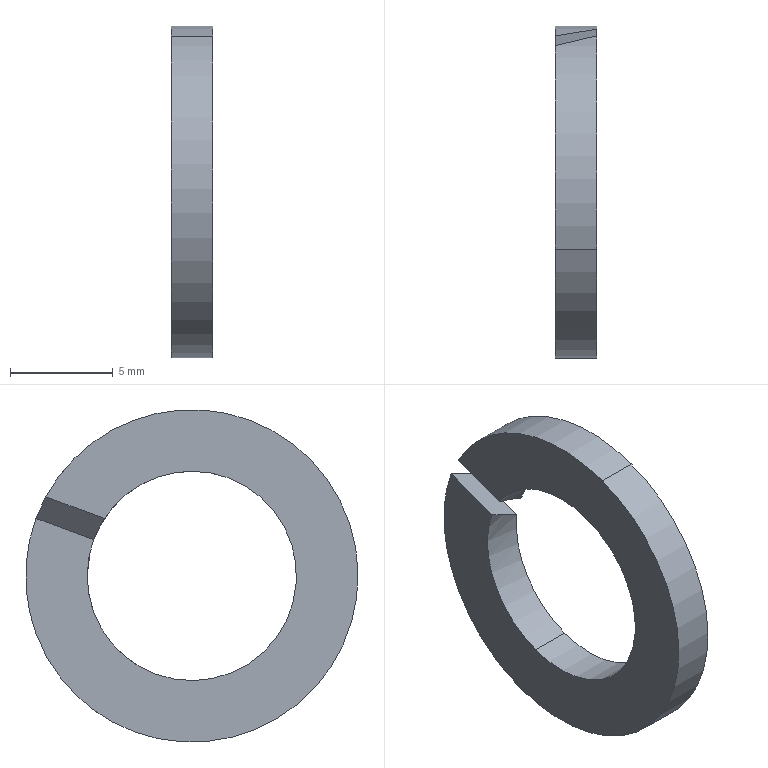Part | SolidWorks | features BaseBody 1 | 1 solid | 10 faces | box 2 x 16.2 x 16.2 mm | volume 241.867 mm3 | cylinder 6 | plane 4 | commonest cylinder face diameters 10.2 x3 16.2 x3
STEP:
#1=CARTESIAN_POINT('',(456.1,149.784,-28.234));
#2=VERTEX_POINT('',#1);
#3=CARTESIAN_POINT('',(456.1,146.766,-34.784));
#4=VERTEX_POINT('',#3);
#5=CARTESIAN_POINT('',(456.1,145.,-30.));
#6=DIRECTION('',(-1.,0.,0.));
#7=DIRECTION('',(0.,-0.3463,0.9381));
#8=AXIS2_PLACEMENT_3D('',#5,#6,#7);
#9=CIRCLE('',#8,5.1);
#10=EDGE_CURVE('',#2,#4,#9,.T.);
#11=ORIENTED_EDGE('',*,*,#10,.T.);
#12=CARTESIAN_POINT('',(458.1,146.766,-34.784));
#13=VERTEX_POINT('',#12);
#14=CARTESIAN_POINT('',(456.1,146.766,-34.784));
#15=DIRECTION('',(1.,0.,0.));
#16=VECTOR('',#15,1000.);
#17=LINE('',#14,#16);
#18=EDGE_CURVE('',#4,#13,#17,.T.);
#19=ORIENTED_EDGE('',*,*,#18,.T.);
#20=CARTESIAN_POINT('',(458.1,150.06,-29.363));
#21=VERTEX_POINT('',#20);
#22=CARTESIAN_POINT('',(458.1,145.,-30.));
#23=DIRECTION('',(-1.,0.,0.));
#24=DIRECTION('',(0.,0.3463,-0.9381));
#25=AXIS2_PLACEMENT_3D('',#22,#23,#24);
#26=CIRCLE('',#25,5.1);
#27=EDGE_CURVE('',#21,#13,#26,.T.);
#28=ORIENTED_EDGE('',*,*,#27,.F.);
#29=CARTESIAN_POINT('',(458.1,150.06,-29.363));
#30=CARTESIAN_POINT('',(457.444,150.011,-28.977));
#31=CARTESIAN_POINT('',(456.774,149.919,-28.599));
#32=CARTESIAN_POINT('',(456.1,149.784,-28.234));
#33=(BOUNDED_CURVE()B_SPLINE_CURVE(3,(#29,#30,#31,#32),.UNSPECIFIED.,.F.,.T.)B_SPLINE_CURVE_WITH_KNOTS((4,4),(1.342,1.571),.UNSPECIFIED.)CURVE()GEOMETRIC_REPRESENTATION_ITEM()RATIONAL_B_SPLINE_CURVE((1.,0.9957,0.9957,1.))REPRESENTATION_ITEM(''));
#34=EDGE_CURVE('',#21,#2,#33,.T.);
#35=ORIENTED_EDGE('',*,*,#34,.T.);
#36=EDGE_LOOP('',(#11,#19,#28,#35));
#37=FACE_OUTER_BOUND('',#36,.T.);
#38=CARTESIAN_POINT('',(456.1,145.,-30.));
#39=DIRECTION('',(1.,0.,0.));
#40=DIRECTION('',(0.,-0.3463,0.9381));
#41=AXIS2_PLACEMENT_3D('',#38,#39,#40);
#42=CYLINDRICAL_SURFACE('',#41,5.1);
#43=ADVANCED_FACE('',(#37),#42,.F.);
#44=ORIENTED_EDGE('',*,*,#18,.F.);
#45=CARTESIAN_POINT('',(456.1,143.234,-25.216));
#46=VERTEX_POINT('',#45);
#47=CARTESIAN_POINT('',(456.1,145.,-30.));
#48=DIRECTION('',(-1.,0.,0.));
#49=DIRECTION('',(0.,-0.3463,0.9381));
#50=AXIS2_PLACEMENT_3D('',#47,#48,#49);
#51=CIRCLE('',#50,5.1);
#52=EDGE_CURVE('',#4,#46,#51,.T.);
#53=ORIENTED_EDGE('',*,*,#52,.T.);
#54=CARTESIAN_POINT('',(458.1,143.234,-25.216));
#55=VERTEX_POINT('',#54);
#56=CARTESIAN_POINT('',(456.1,143.234,-25.216));
#57=DIRECTION('',(1.,0.,0.));
#58=VECTOR('',#57,1000.);
#59=LINE('',#56,#58);
#60=EDGE_CURVE('',#46,#55,#59,.T.);
#61=ORIENTED_EDGE('',*,*,#60,.T.);
#62=CARTESIAN_POINT('',(458.1,145.,-30.));
#63=DIRECTION('',(-1.,0.,0.));
#64=DIRECTION('',(0.,0.3463,-0.9381));
#65=AXIS2_PLACEMENT_3D('',#62,#63,#64);
#66=CIRCLE('',#65,5.1);
#67=EDGE_CURVE('',#13,#55,#66,.T.);
#68=ORIENTED_EDGE('',*,*,#67,.F.);
#69=EDGE_LOOP('',(#44,#53,#61,#68));
#70=FACE_OUTER_BOUND('',#69,.T.);
#71=CARTESIAN_POINT('',(456.1,145.,-30.));
#72=DIRECTION('',(1.,0.,0.));
#73=DIRECTION('',(0.,-0.3463,0.9381));
#74=AXIS2_PLACEMENT_3D('',#71,#72,#73);
#75=CYLINDRICAL_SURFACE('',#74,5.1);
#76=ADVANCED_FACE('',(#70),#75,.F.);
#77=CARTESIAN_POINT('',(456.1,147.805,-37.599));
#78=VERTEX_POINT('',#77);
#79=CARTESIAN_POINT('',(456.1,142.195,-22.401));
#80=VERTEX_POINT('',#79);
#81=CARTESIAN_POINT('',(456.1,145.,-30.));
#82=DIRECTION('',(-1.,0.,0.));
#83=DIRECTION('',(0.,-0.3463,0.9381));
#84=AXIS2_PLACEMENT_3D('',#81,#82,#83);
#85=CIRCLE('',#84,8.1);
#86=EDGE_CURVE('',#78,#80,#85,.T.);
#87=ORIENTED_EDGE('',*,*,#86,.F.);
#88=CARTESIAN_POINT('',(458.1,147.805,-37.599));
#89=VERTEX_POINT('',#88);
#90=CARTESIAN_POINT('',(456.1,147.805,-37.599));
#91=DIRECTION('',(1.,0.,0.));
#92=VECTOR('',#91,1000.);
#93=LINE('',#90,#92);
#94=EDGE_CURVE('',#78,#89,#93,.T.);
#95=ORIENTED_EDGE('',*,*,#94,.T.);
#96=CARTESIAN_POINT('',(458.1,142.195,-22.401));
#97=VERTEX_POINT('',#96);
#98=CARTESIAN_POINT('',(458.1,145.,-30.));
#99=DIRECTION('',(-1.,0.,0.));
#100=DIRECTION('',(0.,0.3463,-0.9381));
#101=AXIS2_PLACEMENT_3D('',#98,#99,#100);
#102=CIRCLE('',#101,8.1);
#103=EDGE_CURVE('',#89,#97,#102,.T.);
#104=ORIENTED_EDGE('',*,*,#103,.T.);
#105=CARTESIAN_POINT('',(456.1,142.195,-22.401));
#106=DIRECTION('',(1.,0.,0.));
#107=VECTOR('',#106,1000.);
#108=LINE('',#105,#107);
#109=EDGE_CURVE('',#80,#97,#108,.T.);
#110=ORIENTED_EDGE('',*,*,#109,.F.);
#111=EDGE_LOOP('',(#87,#95,#104,#110));
#112=FACE_OUTER_BOUND('',#111,.T.);
#113=CARTESIAN_POINT('',(456.1,145.,-30.));
#114=DIRECTION('',(1.,0.,0.));
#115=DIRECTION('',(0.,-0.3463,0.9381));
#116=AXIS2_PLACEMENT_3D('',#113,#114,#115);
#117=CYLINDRICAL_SURFACE('',#116,8.1);
#118=ADVANCED_FACE('',(#112),#117,.T.);
#119=CARTESIAN_POINT('',(456.1,152.121,-26.14));
#120=VERTEX_POINT('',#119);
#121=CARTESIAN_POINT('',(456.1,145.,-30.));
#122=DIRECTION('',(-1.,0.,0.));
#123=DIRECTION('',(0.,-0.3463,0.9381));
#124=AXIS2_PLACEMENT_3D('',#121,#122,#123);
#125=CIRCLE('',#124,8.1);
#126=EDGE_CURVE('',#80,#120,#125,.T.);
#127=ORIENTED_EDGE('',*,*,#126,.F.);
#128=ORIENTED_EDGE('',*,*,#109,.T.);
#129=CARTESIAN_POINT('',(458.1,152.599,-27.195));
#130=VERTEX_POINT('',#129);
#131=CARTESIAN_POINT('',(458.1,145.,-30.));
#132=DIRECTION('',(-1.,0.,0.));
#133=DIRECTION('',(0.,0.3463,-0.9381));
#134=AXIS2_PLACEMENT_3D('',#131,#132,#133);
#135=CIRCLE('',#134,8.1);
#136=EDGE_CURVE('',#97,#130,#135,.T.);
#137=ORIENTED_EDGE('',*,*,#136,.T.);
#138=CARTESIAN_POINT('',(456.1,152.121,-26.14));
#139=CARTESIAN_POINT('',(456.763,152.305,-26.48));
#140=CARTESIAN_POINT('',(457.43,152.465,-26.832));
#141=CARTESIAN_POINT('',(458.1,152.599,-27.195));
#142=(BOUNDED_CURVE()B_SPLINE_CURVE(3,(#138,#139,#140,#141),.UNSPECIFIED.,.F.,.F.)B_SPLINE_CURVE_WITH_KNOTS((4,4),(4.569,4.712),.UNSPECIFIED.)CURVE()GEOMETRIC_REPRESENTATION_ITEM()RATIONAL_B_SPLINE_CURVE((1.,0.9983,0.9983,1.))REPRESENTATION_ITEM(''));
#143=EDGE_CURVE('',#120,#130,#142,.T.);
#144=ORIENTED_EDGE('',*,*,#143,.F.);
#145=EDGE_LOOP('',(#127,#128,#137,#144));
#146=FACE_OUTER_BOUND('',#145,.T.);
#147=CARTESIAN_POINT('',(456.1,145.,-30.));
#148=DIRECTION('',(1.,0.,0.));
#149=DIRECTION('',(0.,-0.3463,0.9381));
#150=AXIS2_PLACEMENT_3D('',#147,#148,#149);
#151=CYLINDRICAL_SURFACE('',#150,8.1);
#152=ADVANCED_FACE('',(#146),#151,.T.);
#153=ORIENTED_EDGE('',*,*,#10,.F.);
#154=CARTESIAN_POINT('',(456.1,152.599,-27.195));
#155=VERTEX_POINT('',#154);
#156=CARTESIAN_POINT('',(456.1,152.6,-27.194));
#157=DIRECTION('',(0.,-0.9381,-0.3463));
#158=VECTOR('',#157,1000.);
#159=LINE('',#156,#158);
#160=EDGE_CURVE('',#155,#2,#159,.T.);
#161=ORIENTED_EDGE('',*,*,#160,.F.);
#162=CARTESIAN_POINT('',(456.1,145.,-30.));
#163=DIRECTION('',(-1.,0.,0.));
#164=DIRECTION('',(0.,-0.3463,0.9381));
#165=AXIS2_PLACEMENT_3D('',#162,#163,#164);
#166=CIRCLE('',#165,8.1);
#167=EDGE_CURVE('',#155,#78,#166,.T.);
#168=ORIENTED_EDGE('',*,*,#167,.T.);
#169=ORIENTED_EDGE('',*,*,#86,.T.);
#170=ORIENTED_EDGE('',*,*,#126,.T.);
#171=CARTESIAN_POINT('',(456.1,149.26,-27.196));
#172=VERTEX_POINT('',#171);
#173=CARTESIAN_POINT('',(456.1,152.2,-26.111));
#174=DIRECTION('',(0.,-0.9381,-0.3463));
#175=VECTOR('',#174,1000.);
#176=LINE('',#173,#175);
#177=EDGE_CURVE('',#120,#172,#176,.T.);
#178=ORIENTED_EDGE('',*,*,#177,.T.);
#179=CARTESIAN_POINT('',(456.1,145.,-30.));
#180=DIRECTION('',(-1.,0.,0.));
#181=DIRECTION('',(0.,-0.3463,0.9381));
#182=AXIS2_PLACEMENT_3D('',#179,#180,#181);
#183=CIRCLE('',#182,5.1);
#184=EDGE_CURVE('',#46,#172,#183,.T.);
#185=ORIENTED_EDGE('',*,*,#184,.F.);
#186=ORIENTED_EDGE('',*,*,#52,.F.);
#187=EDGE_LOOP('',(#153,#161,#168,#169,#170,#178,#185,#186));
#188=FACE_OUTER_BOUND('',#187,.T.);
#189=CARTESIAN_POINT('',(456.1,145.,-30.));
#190=DIRECTION('',(1.,0.,0.));
#191=DIRECTION('',(0.,-0.3463,0.9381));
#192=AXIS2_PLACEMENT_3D('',#189,#190,#191);
#193=PLANE('',#192);
#194=ADVANCED_FACE('',(#188),#193,.F.);
#195=CARTESIAN_POINT('',(458.1,152.921,-28.306));
#196=VERTEX_POINT('',#195);
#197=CARTESIAN_POINT('',(458.1,153.,-28.277));
#198=DIRECTION('',(0.,-0.9381,-0.3463));
#199=VECTOR('',#198,1000.);
#200=LINE('',#197,#199);
#201=EDGE_CURVE('',#196,#21,#200,.T.);
#202=ORIENTED_EDGE('',*,*,#201,.T.);
#203=ORIENTED_EDGE('',*,*,#27,.T.);
#204=ORIENTED_EDGE('',*,*,#67,.T.);
#205=CARTESIAN_POINT('',(458.1,149.784,-28.234));
#206=VERTEX_POINT('',#205);
#207=CARTESIAN_POINT('',(458.1,145.,-30.));
#208=DIRECTION('',(-1.,0.,0.));
#209=DIRECTION('',(0.,0.3463,-0.9381));
#210=AXIS2_PLACEMENT_3D('',#207,#208,#209);
#211=CIRCLE('',#210,5.1);
#212=EDGE_CURVE('',#55,#206,#211,.T.);
#213=ORIENTED_EDGE('',*,*,#212,.T.);
#214=CARTESIAN_POINT('',(458.1,152.6,-27.194));
#215=DIRECTION('',(0.,-0.9381,-0.3463));
#216=VECTOR('',#215,1000.);
#217=LINE('',#214,#216);
#218=EDGE_CURVE('',#130,#206,#217,.T.);
#219=ORIENTED_EDGE('',*,*,#218,.F.);
#220=ORIENTED_EDGE('',*,*,#136,.F.);
#221=ORIENTED_EDGE('',*,*,#103,.F.);
#222=CARTESIAN_POINT('',(458.1,145.,-30.));
#223=DIRECTION('',(-1.,0.,0.));
#224=DIRECTION('',(0.,0.3463,-0.9381));
#225=AXIS2_PLACEMENT_3D('',#222,#223,#224);
#226=CIRCLE('',#225,8.1);
#227=EDGE_CURVE('',#196,#89,#226,.T.);
#228=ORIENTED_EDGE('',*,*,#227,.F.);
#229=EDGE_LOOP('',(#202,#203,#204,#213,#219,#220,#221,#228));
#230=FACE_OUTER_BOUND('',#229,.T.);
#231=CARTESIAN_POINT('',(458.1,145.,-30.));
#232=DIRECTION('',(1.,0.,0.));
#233=DIRECTION('',(0.,-0.3463,0.9381));
#234=AXIS2_PLACEMENT_3D('',#231,#232,#233);
#235=PLANE('',#234);
#236=ADVANCED_FACE('',(#230),#235,.T.);
#237=ORIENTED_EDGE('',*,*,#94,.F.);
#238=ORIENTED_EDGE('',*,*,#167,.F.);
#239=CARTESIAN_POINT('',(458.1,152.921,-28.306));
#240=CARTESIAN_POINT('',(457.437,152.84,-27.928));
#241=CARTESIAN_POINT('',(456.77,152.733,-27.557));
#242=CARTESIAN_POINT('',(456.1,152.599,-27.195));
#243=(BOUNDED_CURVE()B_SPLINE_CURVE(3,(#239,#240,#241,#242),.UNSPECIFIED.,.F.,.F.)B_SPLINE_CURVE_WITH_KNOTS((4,4),(1.428,1.571),.UNSPECIFIED.)CURVE()GEOMETRIC_REPRESENTATION_ITEM()RATIONAL_B_SPLINE_CURVE((1.,0.9983,0.9983,1.))REPRESENTATION_ITEM(''));
#244=EDGE_CURVE('',#196,#155,#243,.T.);
#245=ORIENTED_EDGE('',*,*,#244,.F.);
#246=ORIENTED_EDGE('',*,*,#227,.T.);
#247=EDGE_LOOP('',(#237,#238,#245,#246));
#248=FACE_OUTER_BOUND('',#247,.T.);
#249=CARTESIAN_POINT('',(456.1,145.,-30.));
#250=DIRECTION('',(1.,0.,0.));
#251=DIRECTION('',(0.,-0.3463,0.9381));
#252=AXIS2_PLACEMENT_3D('',#249,#250,#251);
#253=CYLINDRICAL_SURFACE('',#252,8.1);
#254=ADVANCED_FACE('',(#248),#253,.T.);
#255=ORIENTED_EDGE('',*,*,#60,.F.);
#256=ORIENTED_EDGE('',*,*,#184,.T.);
#257=CARTESIAN_POINT('',(456.1,149.26,-27.196));
#258=CARTESIAN_POINT('',(456.756,149.474,-27.521));
#259=CARTESIAN_POINT('',(457.426,149.65,-27.869));
#260=CARTESIAN_POINT('',(458.1,149.784,-28.234));
#261=(BOUNDED_CURVE()B_SPLINE_CURVE(3,(#257,#258,#259,#260),.UNSPECIFIED.,.F.,.F.)B_SPLINE_CURVE_WITH_KNOTS((4,4),(4.484,4.712),.UNSPECIFIED.)CURVE()GEOMETRIC_REPRESENTATION_ITEM()RATIONAL_B_SPLINE_CURVE((1.,0.9957,0.9957,1.))REPRESENTATION_ITEM(''));
#262=EDGE_CURVE('',#172,#206,#261,.T.);
#263=ORIENTED_EDGE('',*,*,#262,.T.);
#264=ORIENTED_EDGE('',*,*,#212,.F.);
#265=EDGE_LOOP('',(#255,#256,#263,#264));
#266=FACE_OUTER_BOUND('',#265,.T.);
#267=CARTESIAN_POINT('',(456.1,145.,-30.));
#268=DIRECTION('',(1.,0.,0.));
#269=DIRECTION('',(0.,-0.3463,0.9381));
#270=AXIS2_PLACEMENT_3D('',#267,#268,#269);
#271=CYLINDRICAL_SURFACE('',#270,5.1);
#272=ADVANCED_FACE('',(#266),#271,.F.);
#273=ORIENTED_EDGE('',*,*,#143,.T.);
#274=ORIENTED_EDGE('',*,*,#218,.T.);
#275=ORIENTED_EDGE('',*,*,#262,.F.);
#276=ORIENTED_EDGE('',*,*,#177,.F.);
#277=EDGE_LOOP('',(#273,#274,#275,#276));
#278=FACE_OUTER_BOUND('',#277,.T.);
#279=CARTESIAN_POINT('',(456.1,152.2,-26.111));
#280=DIRECTION('',(0.5,-0.2999,0.8124));
#281=DIRECTION('',(-0.866,-0.1732,0.4691));
#282=AXIS2_PLACEMENT_3D('',#279,#280,#281);
#283=PLANE('',#282);
#284=ADVANCED_FACE('',(#278),#283,.F.);
#285=ORIENTED_EDGE('',*,*,#244,.T.);
#286=ORIENTED_EDGE('',*,*,#160,.T.);
#287=ORIENTED_EDGE('',*,*,#34,.F.);
#288=ORIENTED_EDGE('',*,*,#201,.F.);
#289=EDGE_LOOP('',(#285,#286,#287,#288));
#290=FACE_OUTER_BOUND('',#289,.T.);
#291=CARTESIAN_POINT('',(458.1,153.,-28.277));
#292=DIRECTION('',(-0.5,0.2999,-0.8124));
#293=DIRECTION('',(0.866,0.1732,-0.4691));
#294=AXIS2_PLACEMENT_3D('',#291,#292,#293);
#295=PLANE('',#294);
#296=ADVANCED_FACE('',(#290),#295,.F.);
#297=CLOSED_SHELL('',(#43,#76,#118,#152,#194,#236,#254,#272,#284,#296));
#298=MANIFOLD_SOLID_BREP('',#297);
#299=CARTESIAN_POINT('',(0.,0.,0.));
#300=DIRECTION('',(0.,0.,1.));
#301=DIRECTION('',(1.,0.,0.));
#302=AXIS2_PLACEMENT_3D('',#299,#300,#301);
#303=(LENGTH_UNIT()NAMED_UNIT(*)SI_UNIT(.MILLI.,.METRE.));
#304=UNCERTAINTY_MEASURE_WITH_UNIT(LENGTH_MEASURE(0.00001),#303,'','');
#305=(NAMED_UNIT(*)PLANE_ANGLE_UNIT()SI_UNIT($,.RADIAN.));
#306=(NAMED_UNIT(*)SI_UNIT($,.STERADIAN.)SOLID_ANGLE_UNIT());
#307=(GEOMETRIC_REPRESENTATION_CONTEXT(3)GLOBAL_UNCERTAINTY_ASSIGNED_CONTEXT((#304))GLOBAL_UNIT_ASSIGNED_CONTEXT((#303,#305,#306))REPRESENTATION_CONTEXT('',''));
#308=ADVANCED_BREP_SHAPE_REPRESENTATION('',(#298,#302),#307);